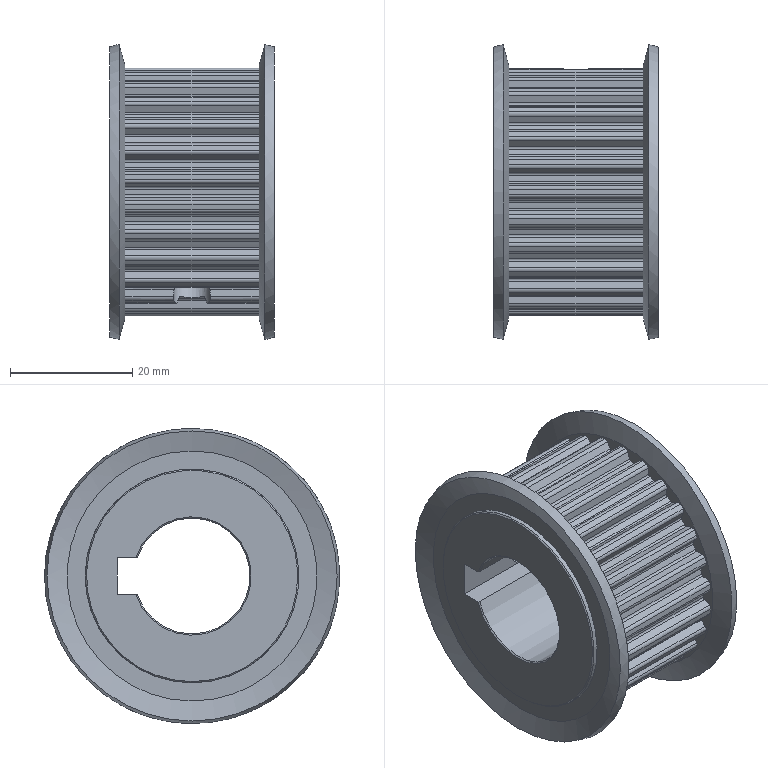Part | NX | 1 solid | 258 faces | box 27 x 48.354 x 48.354 mm | volume 25085 mm3 | cylinder 179 | plane 67 | cone 12 | commonest cylinder face diameters 0.8 x57 1.2 x56 40.6 x29 37 x28 6 x4 4.917 x2